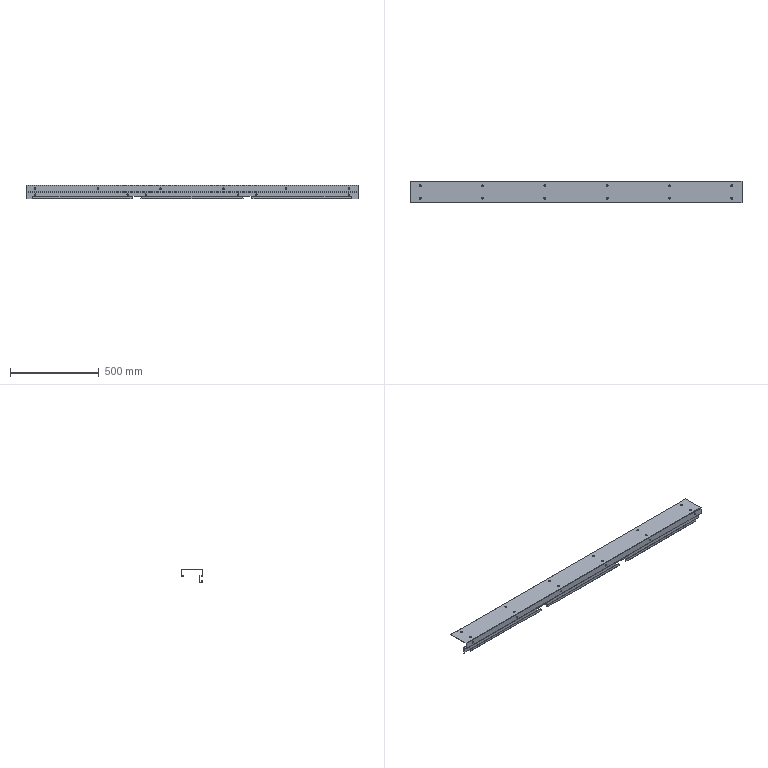Part | STEP file | SX-022-01 | 1 solid | 198 faces | box 1870 x 122 x 78 mm | volume 1056252 mm3 | plane 108 | cylinder 90 | commonest cylinder face diameters 8 x24 10 x24 0.4 x13 4.4 x13 5.4 x12 20 x4